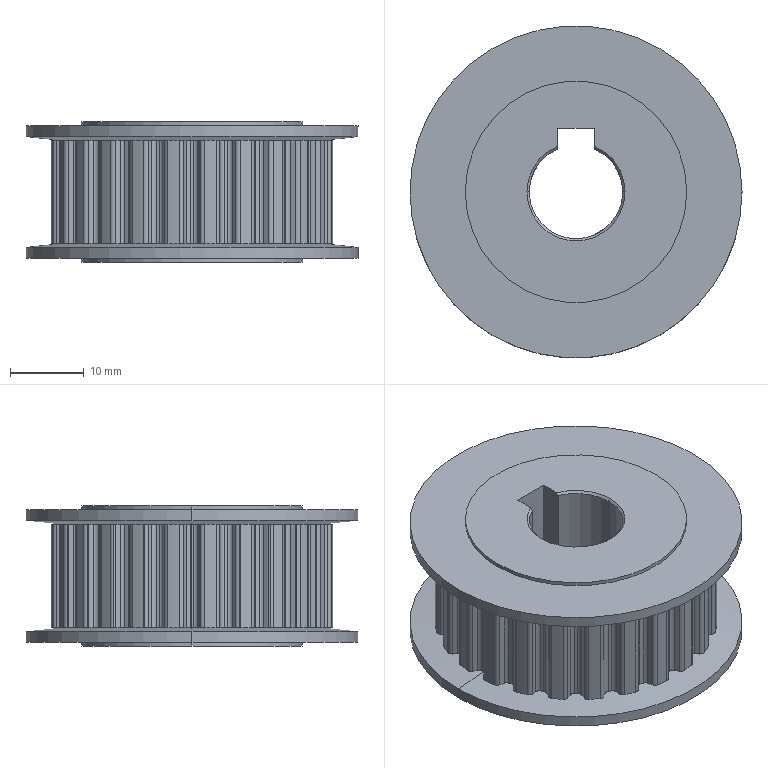Part | STEP file | EAF51-XL050-24-A-N-d12_7 | 1 solid | 369 faces | box 45 x 45 x 19 mm | volume 19278 mm3 | cylinder 182 | plane 173 | cone 14 | commonest cylinder face diameters 1.22 x116 35.5 x27 38.3 x24 4.134 x4 30 x4 45 x4